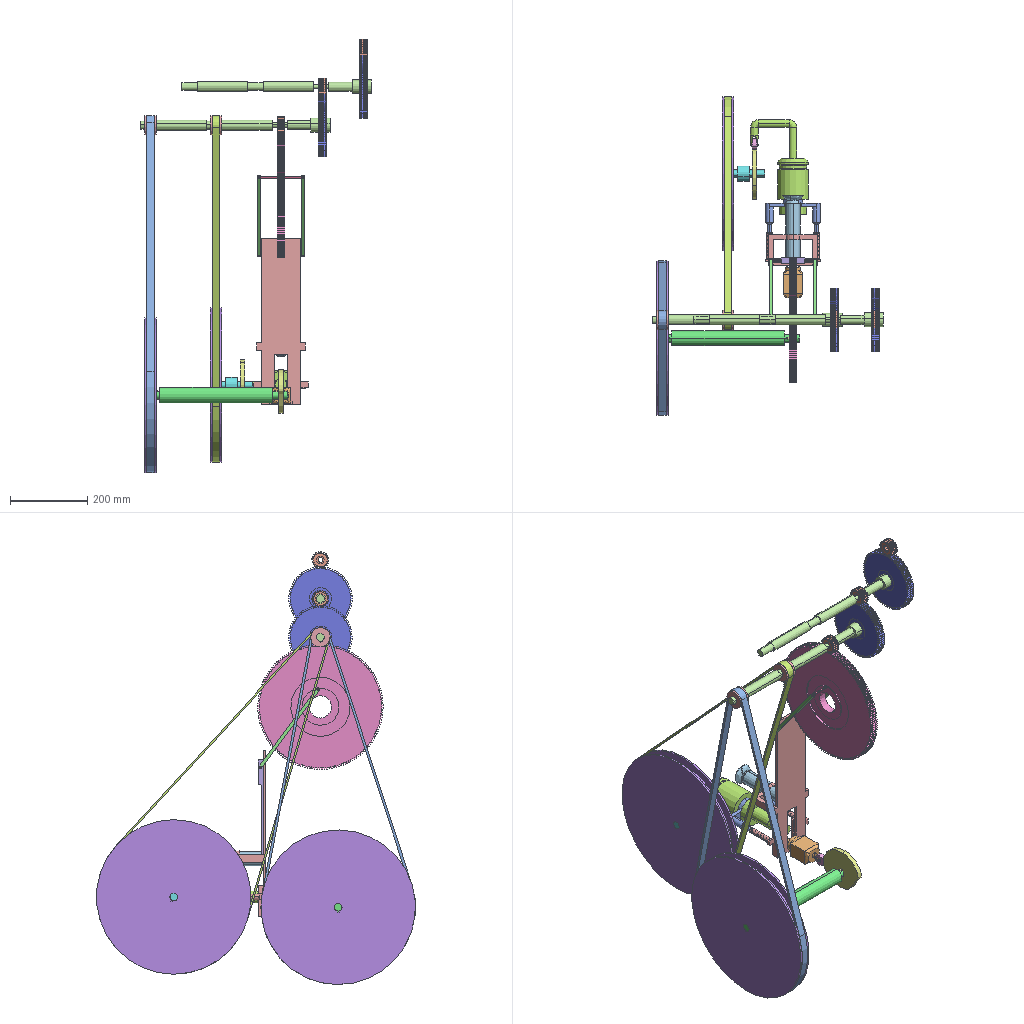Assembly | SolidWorks | 31 different items | 50 placed | box 597 x 824 x 1120 mm
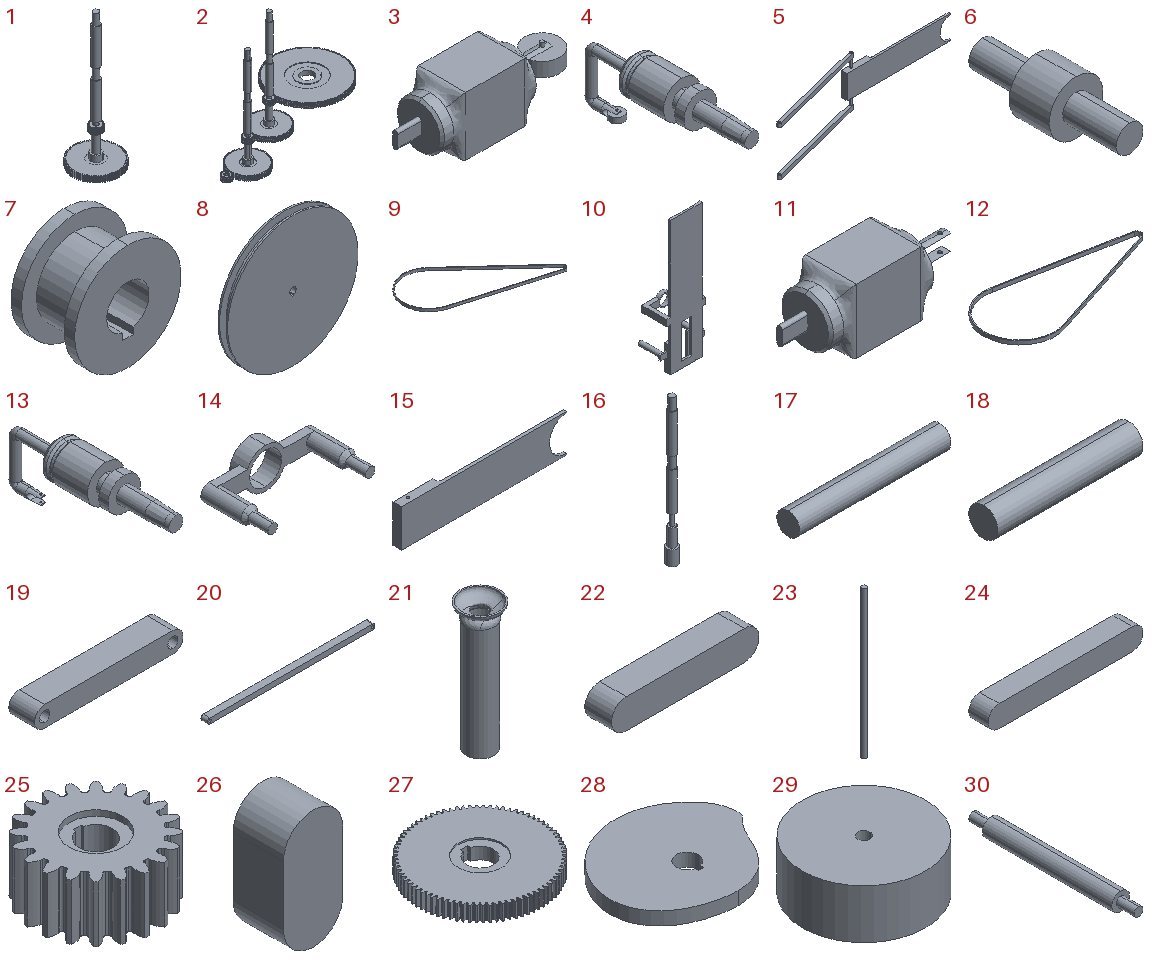Parts list (item | name | quantity | parent item | size | volume | features):
1 | (subassembly) | x2 | in 2 | 163.961 x 163.961 x 490 mm | 641147 mm3 | features RefAxis 2
2 | (subassembly) | x1 | - | 563.839 x 324 x 596.9 mm | 2766981 mm3 | features CompositeCurve 6, RefAxis 4, AEMSimFeature 1
3 | (subassembly) | x1 | - | 140 x 40 x 50 mm | 155331 mm3 | -
4 | (subassembly) | x1 | - | 80 x 358 x 150 mm | 794791 mm3 | -
5 | (subassembly) | x1 | - | 491.967 x 70.667 x 124 mm | 148727 mm3 | features AEMSimFeature 1
6 | - | x1 | - | 40 x 110 x 40 mm | 62258 mm3 | features ICE 1, MirrorPattern 1, Revolution 1
7 | - | x2 | - | 50 x 30 x 50 mm | 30150 mm3 | features ICE 1, Revolution 1
8 | - | x2 | - | 400 x 30 x 400 mm | 3282546 mm3 | features ICE 1, Revolution 1
9 | - | x1 | - | 896.88 x 604.508 x 20 mm | 200125 mm3 | features Sweep 1
10 | - | x1 | - | 142 x 88.365 x 430 mm | 380950 mm3 | features ICE 9, BossThin 2, MirrorPattern 2, Extrusion 1, Helix 1, RefPoint 1, Sweep 1
11 | - | x1 | in 3 | 130 x 40 x 50 mm | 146792 mm3 | features ICE 7, Blend 2, Chamfer 1, Extrusion 1, RefAxis 1, Revolution 1
12 | - | x1 | - | 923.5 x 400 x 20 mm | 251339 mm3 | features Sweep 1
13 | - | x1 | in 4 | 80 x 358 x 150 mm | 786252 mm3 | features ICE 10, Chamfer 3, Extrusion 1, RefAxis 1, Revolution 1, Sweep 1
14 | - | x1 | - | 142.002 x 90 x 50 mm | 64913 mm3 | features ICE 3, Blend 2, ExtruThin 1
15 | - | x1 | in 5 | 263.439 x 13.991 x 60 mm | 106666 mm3 | features ICE 2, Extrusion 1, Fillet 1
16 | - | x2 | in 1 | 36 x 36 x 490 mm | 244254 mm3 | features ICE 6, Extrusion 1, Revolution 1
17 | - | x2 | in 3, 4 | 20 x 3 x 3 mm | 141.372 mm3 | features Extrusion 1
18 | - | x1 | in 5 | 20 x 4 x 4 mm | 251.327 mm3 | features Extrusion 1
19 | - | x1 | in 5 | 58 x 10 x 8 mm | 4251 mm3 | features Extrusion 1
20 | - | x2 | in 5 | 258 x 10 x 8 mm | 20251 mm3 | features Extrusion 1
21 | - | x1 | - | 53.043 x 53.043 x 170 mm | 40176 mm3 | features Blend 1, ExtruThin 1
22 | - | x6 | - | 25 x 4.5 x 5 mm | 538.357 mm3 | features Extrusion 1
23 | - | x2 | in 5 | 4 x 4 x 124 mm | 1558 mm3 | features Extrusion 1
24 | - | x2 | in 1 | 20 x 2.5 x 2.8 mm | 135.794 mm3 | features Extrusion 1
25 | - | x3 | in 1, 2 | 43.654 x 43.654 x 20 mm | 21667 mm3 | features ICE 4, Extrusion 1
26 | - | x2 | in 1 | 10 x 8.5 x 20 mm | 1518 mm3 | features Extrusion 1
27 | - | x2 | in 1 | 163.929 x 163.929 x 20 mm | 373573 mm3 | features ICE 4, Extrusion 1
28 | - | x2 | - | 127.495 x 112.48 x 12 mm | 126053 mm3 | features Extrusion 1
29 | - | x2 | in 3, 4 | 30 x 30 x 12 mm | 8397 mm3 | features Extrusion 1
30 | - | x1 | - | 40 x 370 x 40 mm | 388983 mm3 | features ICE 1, MirrorPattern 1, Revolution 1
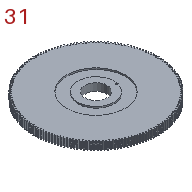31 | - | x1 | in 2 | 323.966 x 323.966 x 20 mm | 1463021 mm3 | features ICE 5, Cut 1, Extrusion 1
Mates (type | each side: item.copy, entity, surface, feature):
In the top assembly
Concentric | 10.1 face cylinder Extrude-Thin1 | 14.1 face cylinder Boss-Extrude4 | 2 times
Coincident | 14.1 face plane Extrude-Thin1 | 13.1 face plane Boss-Extrude4
Concentric | 14.1 face cylinder Extrude-Thin1 | 13.1 face cylinder Boss-Extrude5
DistanceDim | 11.1 face plane Boss-Extrude5 | 10.1 face plane Cut-Extrude4
Coincident | 10.1 plane | 3.1 plane
Coincident | 10.1 face plane Cut-Extrude3 | 15.1 face plane Boss-Extrude2
Coincident | 10.1 plane | 15.1 plane
Concentric | 10.1 face cylinder Extrude-Thin2 | 21.1 face cylinder Extrude-Thin1
Coincident | 10.1 plane | 13.1 plane
Coincident | 29.1 face plane Boss-Extrude1 | 28.1 face plane Boss-Extrude1
Concentric | 31.1 face cylinder Cut-Extrude3 | assembly select_type:11
Coincident | 10.1 plane | 31.1 plane
Parallel | 10.1 plane | 2.1 plane
Concentric | 6.1 face cylinder Cut-Extrude1 | 22.1 face cylinder Boss-Extrude1
Coincident | 6.1 face plane Cut-Extrude1 | 22.1 face plane Boss-Extrude1 | 2 times
Coincident | 30.1 face plane Cut-Extrude1 | 22.2 face plane Boss-Extrude1 | 2 times
Concentric | 30.1 face cylinder Cut-Extrude1 | 22.2 face cylinder Boss-Extrude1
Coincident | 30.1 face plane Mirror1 | 22.3 face plane Boss-Extrude1 | 2 times
Concentric | 30.1 face cylinder Mirror1 | 22.3 face cylinder Boss-Extrude1
Concentric | 28.1 face cylinder Boss-Extrude1 | 30.1 face cylinder Revolve1
Coincident | 28.1 face plane Boss-Extrude1 | 22.3 face plane Boss-Extrude1
Coincident | 8.1 face plane Cut-Extrude1 | 22.2 face plane Boss-Extrude1
Coincident | 16.1 face plane Revolve1 | 8.1 face plane Revolve1
Coincident | 16.1 face plane Revolve1 | 8.2 face plane Revolve1
Coincident | 16.1 face plane Cut-Extrude6 | 22.4 face plane Boss-Extrude1 | 2 times
Concentric | 16.1 face cylinder Cut-Extrude6 | 22.4 face cylinder Boss-Extrude1
Coincident | 16.1 face plane Cut-Extrude5 | 22.5 face plane Boss-Extrude1 | 2 times
Concentric | 16.1 face cylinder Cut-Extrude5 | 22.5 face cylinder Boss-Extrude1
Coincident | 7.1 face plane Cut-Extrude1 | 22.5 face plane Boss-Extrude1
Concentric | 16.1 face cylinder Revolve1 | 7.1 face cylinder Revolve1
Coincident | 16.1 face plane Revolve1 | 7.1 face plane Revolve1
Coincident | 7.2 face plane Cut-Extrude1 | 22.4 face plane Boss-Extrude1
Concentric | 16.1 face cylinder Revolve1 | 7.2 face cylinder Revolve1
Coincident | 16.1 face plane Revolve1 | 7.2 face plane Revolve1
Concentric | 20.1 face cylinder Boss-Extrude1 | 31.1 face cylinder Cut-Extrude5
Concentric | 31.1 face cylinder Cut-Extrude5 | 23.1 face cylinder Boss-Extrude1
Coincident | 20.2 face plane Boss-Extrude1 | 23.1 face plane Boss-Extrude1
Concentric | 8.1 face cylinder Revolve1 | 30.1 face cylinder Revolve1
Coincident | 6.1 face plane Mirror1 | 22.6 face plane Boss-Extrude1 | 2 times
Concentric | 6.1 face cylinder Mirror1 | 22.6 face cylinder Boss-Extrude1
Concentric | 28.2 face cylinder Boss-Extrude1 | 6.1 face cylinder Revolve1
Coincident | 28.2 face plane Boss-Extrude1 | 22.6 face plane Boss-Extrude1
CamTangent | 28.2 face surface:4009 Boss-Extrude1 | 29.2 face cylinder Boss-Extrude1
Coincident | 29.2 face plane Boss-Extrude1 | 28.2 face plane Boss-Extrude1
Concentric | 6.1 face cylinder Revolve1 | 8.2 face cylinder Revolve1
Coincident | 22.1 face plane Boss-Extrude1 | 8.2 face plane Cut-Extrude1
Coincident | 6.1 face plane Revolve1 | 8.2 face plane Revolve1
Concentric | 30.1 face cylinder Revolve1 | assembly axis
Concentric | 6.1 face cylinder Revolve1 | assembly axis
Coincident | 8.1 face plane Revolve1 | 30.1 face plane Revolve1
Concentric | 7.2 face cylinder Revolve1 | 12.1 face cylinder Sweep1
Concentric | 8.1 face cylinder Revolve1 | 12.1 face cylinder Sweep1
Coincident | 8.1 face plane Revolve1 | 12.1 face plane Sweep1
Concentric | 7.1 face cylinder Revolve1 | 9.1 face cylinder Sweep1
Concentric | 8.2 face cylinder Revolve1 | 9.1 face cylinder Sweep1
Coincident | 8.2 face plane Revolve1 | 9.1 face plane Sweep1
Concentric | 25.1 face cylinder Cut-Extrude4 | assembly axis
Concentric | 16.2 face cylinder Boss-Extrude2 | assembly axis
LimitDistanceDim | 10.1 face plane Boss-Extrude1 | 11.1 face plane Boss-Extrude5
GearDim | 8.1 edge | 7.2 edge
GearDim | 8.2 edge | 7.1 edge
Tangent | 29.1 face cylinder Boss-Extrude1 | 28.1 face surface:4009 Boss-Extrude1
In subassembly 2
Concentric | 16.3 face cylinder Boss-Extrude6 | 2.2 axis
Coincident | 27.1 face plane Boss-Extrude1 | 2.2 plane
Coincident | 25.2 plane | 27.2 plane
Concentric | 16.4 face cylinder Boss-Extrude2 | 2.2 axis
GearDim | 27.2 select_type:24 | 25.2 select_type:24
Concentric | 25.3 face cylinder Cut-Extrude4 | 2.2 axis
Coincident | 27.1 plane | 25.3 plane
GearDim | 25.3 select_type:24 | 27.1 select_type:24
Coincident | 25.4 plane | 31.2 plane
Concentric | 31.2 face cylinder Cut-Extrude3 | 2.2 axis
GearDim | 31.2 select_type:24 | 25.4 select_type:24
In subassembly 1
Coincident | 26.1 plane | 16.5 plane
Coincident | 26.1 face plane Boss-Extrude1 | 16.5 face plane Cut-Extrude3
Concentric | 26.1 face cylinder Boss-Extrude1 | 16.5 face cylinder Cut-Extrude3
Coincident | 24.1 plane | 16.5 plane
Coincident | 24.1 face plane Boss-Extrude1 | 16.5 face plane Cut-Extrude4
Concentric | 24.1 face cylinder Boss-Extrude1 | 16.5 face cylinder Cut-Extrude4
Coincident | 26.1 face plane Boss-Extrude1 | 27.3 face plane Cut-Extrude4 | 2 times
Coincident | 26.1 plane | 27.3 plane
Coincident | 24.1 plane | 25.3 plane
Concentric | 16.5 face cylinder Boss-Extrude2 | 1.1 axis
Coincident | 16.5 face plane Boss-Extrude2 | 1.1 plane
Concentric | 25.3 face cylinder Cut-Extrude4 | 16.5 face cylinder Boss-Extrude7
Coincident | 24.1 face plane Boss-Extrude1 | 25.3 face plane Cut-Extrude5
In subassembly 4
Concentric | 13.2 face cylinder Cut-Extrude2 | 29.3 face cylinder Boss-Extrude1
Coincident | 13.2 face plane Cut-Extrude1 | 29.3 face plane Boss-Extrude1
Concentric | 13.2 face cylinder Cut-Extrude2 | 17.1 face cylinder Boss-Extrude1
DistanceDim | 17.1 face plane Boss-Extrude1 | 29.3 face plane Boss-Extrude1
In subassembly 3
Concentric | 11.2 face cylinder Cut-Extrude2 | 29.3 face cylinder Boss-Extrude1
Coincident | 11.2 face plane Cut-Extrude1 | 29.3 face plane Boss-Extrude1
Concentric | 29.3 face cylinder Boss-Extrude1 | 17.1 face cylinder Boss-Extrude1
Lock | 29.3 select_type:0 | 17.1 select_type:0
In subassembly 5
Concentric | 18.1 face | 19.1 edge
Coincident | 19.1 face | 5.1 plane
Coincident | 19.1 face | 20.3 face plane Boss-Extrude1
Coincident | 15.2 plane | 5.1 plane
Concentric | 20.3 face cylinder Boss-Extrude1 | 20.4 face cylinder Boss-Extrude1
Coincident | 19.2 face | 20.4 face plane Boss-Extrude1
Concentric | 19.2 face | 20.4 face cylinder Boss-Extrude1
Concentric | 19.1 face | 19.2 face
Concentric | 15.2 face cylinder Cut-Extrude1 | 20.3 face cylinder Boss-Extrude1
Concentric | 15.2 face cylinder Cut-Extrude1 | 20.4 face cylinder Boss-Extrude1
DistanceDim | 15.2 plane | 20.3 face plane Boss-Extrude1
DistanceDim | 20.3 face plane Boss-Extrude1 | 20.4 face plane Boss-Extrude1
Concentric | 15.2 face cylinder Cut-Extrude1 | 23.2 face cylinder Boss-Extrude1
Coincident | 20.4 face plane Boss-Extrude1 | 23.2 face plane Boss-Extrude1
Concentric | 20.3 face cylinder Boss-Extrude1 | 18.1 face
Coincident | 20.3 face plane Boss-Extrude1 | 18.1 face
Concentric | 19.2 face | 18.2 face
Coincident | 19.2 face | 18.2 face